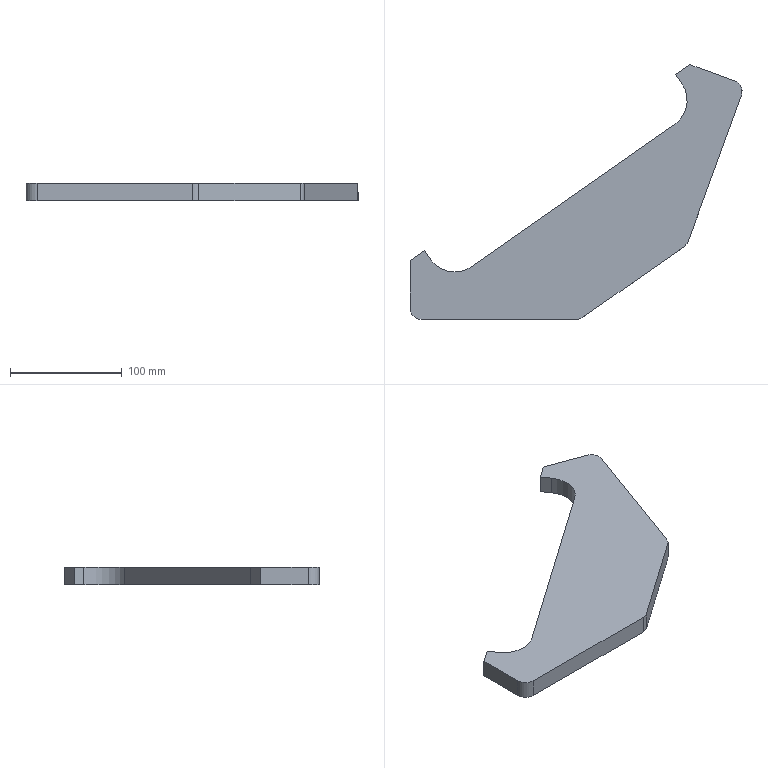Part | SolidWorks | features Extrusion 1, Fillet 1 | 1 solid | 18 faces | box 296.858 x 227.831 x 16 mm | volume 414208 mm3 | plane 12 | cylinder 6 | commonest cylinder face diameters 20 x4 52 x2
STEP:
#1=CARTESIAN_POINT('',(2.583,143.71,16.));
#2=VERTEX_POINT('',#1);
#3=CARTESIAN_POINT('',(93.105,207.095,16.));
#4=VERTEX_POINT('',#3);
#5=CARTESIAN_POINT('',(0.,141.902,16.));
#6=DIRECTION('',(0.8192,0.5736,0.));
#7=VECTOR('',#6,1000.);
#8=LINE('',#5,#7);
#9=EDGE_CURVE('',#2,#4,#8,.T.);
#10=ORIENTED_EDGE('',*,*,#9,.F.);
#11=CARTESIAN_POINT('',(2.583,143.71,0.));
#12=VERTEX_POINT('',#11);
#13=CARTESIAN_POINT('',(2.583,143.71,16.));
#14=DIRECTION('',(0.,0.,-1.));
#15=VECTOR('',#14,1000.);
#16=LINE('',#13,#15);
#17=EDGE_CURVE('',#2,#12,#16,.T.);
#18=ORIENTED_EDGE('',*,*,#17,.T.);
#19=CARTESIAN_POINT('',(93.105,207.095,0.));
#20=VERTEX_POINT('',#19);
#21=CARTESIAN_POINT('',(0.,141.902,0.));
#22=DIRECTION('',(0.8192,0.5736,0.));
#23=VECTOR('',#22,1000.);
#24=LINE('',#21,#23);
#25=EDGE_CURVE('',#12,#20,#24,.T.);
#26=ORIENTED_EDGE('',*,*,#25,.T.);
#27=CARTESIAN_POINT('',(93.105,207.095,16.));
#28=DIRECTION('',(0.,0.,1.));
#29=VECTOR('',#28,1000.);
#30=LINE('',#27,#29);
#31=EDGE_CURVE('',#20,#4,#30,.T.);
#32=ORIENTED_EDGE('',*,*,#31,.T.);
#33=EDGE_LOOP('',(#10,#18,#26,#32));
#34=FACE_OUTER_BOUND('',#33,.T.);
#35=CARTESIAN_POINT('',(0.,141.902,16.));
#36=DIRECTION('',(-0.5736,0.8192,0.));
#37=DIRECTION('',(-0.8192,-0.5736,0.));
#38=AXIS2_PLACEMENT_3D('',#35,#36,#37);
#39=PLANE('',#38);
#40=ADVANCED_FACE('',(#34),#39,.F.);
#41=CARTESIAN_POINT('',(96.767,211.866,16.));
#42=VERTEX_POINT('',#41);
#43=CARTESIAN_POINT('',(144.255,342.34,16.));
#44=VERTEX_POINT('',#43);
#45=CARTESIAN_POINT('',(95.688,208.903,16.));
#46=DIRECTION('',(0.342,0.9397,0.));
#47=VECTOR('',#46,1000.);
#48=LINE('',#45,#47);
#49=EDGE_CURVE('',#42,#44,#48,.T.);
#50=ORIENTED_EDGE('',*,*,#49,.F.);
#51=CARTESIAN_POINT('',(96.767,211.866,0.));
#52=VERTEX_POINT('',#51);
#53=CARTESIAN_POINT('',(96.767,211.866,16.));
#54=DIRECTION('',(0.,0.,-1.));
#55=VECTOR('',#54,1000.);
#56=LINE('',#53,#55);
#57=EDGE_CURVE('',#42,#52,#56,.T.);
#58=ORIENTED_EDGE('',*,*,#57,.T.);
#59=CARTESIAN_POINT('',(144.255,342.34,0.));
#60=VERTEX_POINT('',#59);
#61=CARTESIAN_POINT('',(140.835,332.943,0.));
#62=DIRECTION('',(0.342,0.9397,0.));
#63=VECTOR('',#62,1000.);
#64=LINE('',#61,#63);
#65=EDGE_CURVE('',#52,#60,#64,.T.);
#66=ORIENTED_EDGE('',*,*,#65,.T.);
#67=CARTESIAN_POINT('',(144.255,342.34,16.));
#68=DIRECTION('',(0.,0.,1.));
#69=VECTOR('',#68,1000.);
#70=LINE('',#67,#69);
#71=EDGE_CURVE('',#60,#44,#70,.T.);
#72=ORIENTED_EDGE('',*,*,#71,.T.);
#73=EDGE_LOOP('',(#50,#58,#66,#72));
#74=FACE_OUTER_BOUND('',#73,.T.);
#75=CARTESIAN_POINT('',(140.835,332.943,16.));
#76=DIRECTION('',(-0.9397,0.342,0.));
#77=DIRECTION('',(-0.342,-0.9397,0.));
#78=AXIS2_PLACEMENT_3D('',#75,#76,#77);
#79=PLANE('',#78);
#80=ADVANCED_FACE('',(#74),#79,.F.);
#81=CARTESIAN_POINT('',(138.278,355.157,16.));
#82=VERTEX_POINT('',#81);
#83=CARTESIAN_POINT('',(98.232,369.733,16.));
#84=VERTEX_POINT('',#83);
#85=CARTESIAN_POINT('',(147.675,351.737,16.));
#86=DIRECTION('',(-0.9397,0.342,0.));
#87=VECTOR('',#86,1000.);
#88=LINE('',#85,#87);
#89=EDGE_CURVE('',#82,#84,#88,.T.);
#90=ORIENTED_EDGE('',*,*,#89,.F.);
#91=CARTESIAN_POINT('',(138.278,355.157,0.));
#92=VERTEX_POINT('',#91);
#93=CARTESIAN_POINT('',(138.278,355.157,16.));
#94=DIRECTION('',(0.,0.,-1.));
#95=VECTOR('',#94,1000.);
#96=LINE('',#93,#95);
#97=EDGE_CURVE('',#82,#92,#96,.T.);
#98=ORIENTED_EDGE('',*,*,#97,.T.);
#99=CARTESIAN_POINT('',(98.232,369.733,0.));
#100=VERTEX_POINT('',#99);
#101=CARTESIAN_POINT('',(147.675,351.737,0.));
#102=DIRECTION('',(-0.9397,0.342,0.));
#103=VECTOR('',#102,1000.);
#104=LINE('',#101,#103);
#105=EDGE_CURVE('',#92,#100,#104,.T.);
#106=ORIENTED_EDGE('',*,*,#105,.T.);
#107=CARTESIAN_POINT('',(98.232,369.733,16.));
#108=DIRECTION('',(0.,0.,-1.));
#109=VECTOR('',#108,1000.);
#110=LINE('',#107,#109);
#111=EDGE_CURVE('',#84,#100,#110,.T.);
#112=ORIENTED_EDGE('',*,*,#111,.F.);
#113=EDGE_LOOP('',(#90,#98,#106,#112));
#114=FACE_OUTER_BOUND('',#113,.T.);
#115=CARTESIAN_POINT('',(147.675,351.737,16.));
#116=DIRECTION('',(-0.342,-0.9397,0.));
#117=DIRECTION('',(0.9397,-0.342,0.));
#118=AXIS2_PLACEMENT_3D('',#115,#116,#117);
#119=PLANE('',#118);
#120=ADVANCED_FACE('',(#114),#119,.F.);
#121=CARTESIAN_POINT('',(85.34,360.705,0.));
#122=VERTEX_POINT('',#121);
#123=CARTESIAN_POINT('',(85.34,360.705,0.));
#124=DIRECTION('',(-0.8192,-0.5736,0.));
#125=VECTOR('',#124,1000.);
#126=LINE('',#123,#125);
#127=EDGE_CURVE('',#100,#122,#126,.T.);
#128=ORIENTED_EDGE('',*,*,#127,.T.);
#129=CARTESIAN_POINT('',(85.34,360.705,16.));
#130=VERTEX_POINT('',#129);
#131=CARTESIAN_POINT('',(85.34,360.705,16.));
#132=DIRECTION('',(0.,0.,-1.));
#133=VECTOR('',#132,1000.);
#134=LINE('',#131,#133);
#135=EDGE_CURVE('',#130,#122,#134,.T.);
#136=ORIENTED_EDGE('',*,*,#135,.F.);
#137=CARTESIAN_POINT('',(85.34,360.705,16.));
#138=DIRECTION('',(-0.8192,-0.5736,0.));
#139=VECTOR('',#138,1000.);
#140=LINE('',#137,#139);
#141=EDGE_CURVE('',#84,#130,#140,.T.);
#142=ORIENTED_EDGE('',*,*,#141,.F.);
#143=ORIENTED_EDGE('',*,*,#111,.T.);
#144=EDGE_LOOP('',(#128,#136,#142,#143));
#145=FACE_OUTER_BOUND('',#144,.T.);
#146=CARTESIAN_POINT('',(85.34,360.705,16.));
#147=DIRECTION('',(0.5736,-0.8192,0.));
#148=DIRECTION('',(0.8192,0.5736,0.));
#149=AXIS2_PLACEMENT_3D('',#146,#147,#148);
#150=PLANE('',#149);
#151=ADVANCED_FACE('',(#145),#150,.F.);
#152=CARTESIAN_POINT('',(91.075,352.514,0.));
#153=VERTEX_POINT('',#152);
#154=CARTESIAN_POINT('',(85.34,360.705,0.));
#155=DIRECTION('',(0.5736,-0.8192,0.));
#156=VECTOR('',#155,1000.);
#157=LINE('',#154,#156);
#158=EDGE_CURVE('',#122,#153,#157,.T.);
#159=ORIENTED_EDGE('',*,*,#158,.T.);
#160=CARTESIAN_POINT('',(91.075,352.514,16.));
#161=VERTEX_POINT('',#160);
#162=CARTESIAN_POINT('',(91.075,352.514,16.));
#163=DIRECTION('',(0.,0.,-1.));
#164=VECTOR('',#163,1000.);
#165=LINE('',#162,#164);
#166=EDGE_CURVE('',#161,#153,#165,.T.);
#167=ORIENTED_EDGE('',*,*,#166,.F.);
#168=CARTESIAN_POINT('',(85.34,360.705,16.));
#169=DIRECTION('',(0.5736,-0.8192,0.));
#170=VECTOR('',#169,1000.);
#171=LINE('',#168,#170);
#172=EDGE_CURVE('',#130,#161,#171,.T.);
#173=ORIENTED_EDGE('',*,*,#172,.F.);
#174=ORIENTED_EDGE('',*,*,#135,.T.);
#175=EDGE_LOOP('',(#159,#167,#173,#174));
#176=FACE_OUTER_BOUND('',#175,.T.);
#177=CARTESIAN_POINT('',(85.34,360.705,16.));
#178=DIRECTION('',(0.8192,0.5736,0.));
#179=DIRECTION('',(-0.5736,0.8192,0.));
#180=AXIS2_PLACEMENT_3D('',#177,#178,#179);
#181=PLANE('',#180);
#182=ADVANCED_FACE('',(#176),#181,.F.);
#183=CARTESIAN_POINT('',(84.691,316.303,0.));
#184=VERTEX_POINT('',#183);
#185=CARTESIAN_POINT('',(69.778,337.601,0.));
#186=DIRECTION('',(0.,0.,-1.));
#187=DIRECTION('',(1.,0.,0.));
#188=AXIS2_PLACEMENT_3D('',#185,#186,#187);
#189=CIRCLE('',#188,26.);
#190=EDGE_CURVE('',#153,#184,#189,.T.);
#191=ORIENTED_EDGE('',*,*,#190,.T.);
#192=CARTESIAN_POINT('',(84.691,316.303,16.));
#193=VERTEX_POINT('',#192);
#194=CARTESIAN_POINT('',(84.691,316.303,16.));
#195=DIRECTION('',(0.,0.,-1.));
#196=VECTOR('',#195,1000.);
#197=LINE('',#194,#196);
#198=EDGE_CURVE('',#193,#184,#197,.T.);
#199=ORIENTED_EDGE('',*,*,#198,.F.);
#200=CARTESIAN_POINT('',(69.778,337.601,16.));
#201=DIRECTION('',(0.,0.,-1.));
#202=DIRECTION('',(1.,0.,0.));
#203=AXIS2_PLACEMENT_3D('',#200,#201,#202);
#204=CIRCLE('',#203,26.);
#205=EDGE_CURVE('',#161,#193,#204,.T.);
#206=ORIENTED_EDGE('',*,*,#205,.F.);
#207=ORIENTED_EDGE('',*,*,#166,.T.);
#208=EDGE_LOOP('',(#191,#199,#206,#207));
#209=FACE_OUTER_BOUND('',#208,.T.);
#210=CARTESIAN_POINT('',(69.778,337.601,16.));
#211=DIRECTION('',(0.,0.,-1.));
#212=DIRECTION('',(-1.,0.,0.));
#213=AXIS2_PLACEMENT_3D('',#210,#211,#212);
#214=CYLINDRICAL_SURFACE('',#213,26.);
#215=ADVANCED_FACE('',(#209),#214,.F.);
#216=CARTESIAN_POINT('',(-97.161,188.969,0.));
#217=VERTEX_POINT('',#216);
#218=CARTESIAN_POINT('',(-97.161,188.969,0.));
#219=DIRECTION('',(-0.8192,-0.5736,0.));
#220=VECTOR('',#219,1000.);
#221=LINE('',#218,#220);
#222=EDGE_CURVE('',#184,#217,#221,.T.);
#223=ORIENTED_EDGE('',*,*,#222,.T.);
#224=CARTESIAN_POINT('',(-97.161,188.969,16.));
#225=VERTEX_POINT('',#224);
#226=CARTESIAN_POINT('',(-97.161,188.969,16.));
#227=DIRECTION('',(0.,0.,-1.));
#228=VECTOR('',#227,1000.);
#229=LINE('',#226,#228);
#230=EDGE_CURVE('',#225,#217,#229,.T.);
#231=ORIENTED_EDGE('',*,*,#230,.F.);
#232=CARTESIAN_POINT('',(-97.161,188.969,16.));
#233=DIRECTION('',(-0.8192,-0.5736,0.));
#234=VECTOR('',#233,1000.);
#235=LINE('',#232,#234);
#236=EDGE_CURVE('',#193,#225,#235,.T.);
#237=ORIENTED_EDGE('',*,*,#236,.F.);
#238=ORIENTED_EDGE('',*,*,#198,.T.);
#239=EDGE_LOOP('',(#223,#231,#237,#238));
#240=FACE_OUTER_BOUND('',#239,.T.);
#241=CARTESIAN_POINT('',(-97.161,188.969,16.));
#242=DIRECTION('',(0.5736,-0.8192,0.));
#243=DIRECTION('',(0.8192,0.5736,0.));
#244=AXIS2_PLACEMENT_3D('',#241,#242,#243);
#245=PLANE('',#244);
#246=ADVANCED_FACE('',(#240),#245,.F.);
#247=CARTESIAN_POINT('',(-133.372,195.354,0.));
#248=VERTEX_POINT('',#247);
#249=CARTESIAN_POINT('',(-112.074,210.267,0.));
#250=DIRECTION('',(0.,0.,-1.));
#251=DIRECTION('',(1.,0.,0.));
#252=AXIS2_PLACEMENT_3D('',#249,#250,#251);
#253=CIRCLE('',#252,26.);
#254=EDGE_CURVE('',#217,#248,#253,.T.);
#255=ORIENTED_EDGE('',*,*,#254,.T.);
#256=CARTESIAN_POINT('',(-133.372,195.354,16.));
#257=VERTEX_POINT('',#256);
#258=CARTESIAN_POINT('',(-133.372,195.354,16.));
#259=DIRECTION('',(0.,0.,-1.));
#260=VECTOR('',#259,1000.);
#261=LINE('',#258,#260);
#262=EDGE_CURVE('',#257,#248,#261,.T.);
#263=ORIENTED_EDGE('',*,*,#262,.F.);
#264=CARTESIAN_POINT('',(-112.074,210.267,16.));
#265=DIRECTION('',(0.,0.,-1.));
#266=DIRECTION('',(1.,0.,0.));
#267=AXIS2_PLACEMENT_3D('',#264,#265,#266);
#268=CIRCLE('',#267,26.);
#269=EDGE_CURVE('',#225,#257,#268,.T.);
#270=ORIENTED_EDGE('',*,*,#269,.F.);
#271=ORIENTED_EDGE('',*,*,#230,.T.);
#272=EDGE_LOOP('',(#255,#263,#270,#271));
#273=FACE_OUTER_BOUND('',#272,.T.);
#274=CARTESIAN_POINT('',(-112.074,210.267,16.));
#275=DIRECTION('',(0.,0.,-1.));
#276=DIRECTION('',(-1.,0.,0.));
#277=AXIS2_PLACEMENT_3D('',#274,#275,#276);
#278=CYLINDRICAL_SURFACE('',#277,26.);
#279=ADVANCED_FACE('',(#273),#278,.F.);
#280=CARTESIAN_POINT('',(-139.108,203.546,0.));
#281=VERTEX_POINT('',#280);
#282=CARTESIAN_POINT('',(-133.372,195.354,0.));
#283=DIRECTION('',(-0.5736,0.8192,0.));
#284=VECTOR('',#283,1000.);
#285=LINE('',#282,#284);
#286=EDGE_CURVE('',#248,#281,#285,.T.);
#287=ORIENTED_EDGE('',*,*,#286,.T.);
#288=CARTESIAN_POINT('',(-139.108,203.546,16.));
#289=VERTEX_POINT('',#288);
#290=CARTESIAN_POINT('',(-139.108,203.546,16.));
#291=DIRECTION('',(0.,0.,-1.));
#292=VECTOR('',#291,1000.);
#293=LINE('',#290,#292);
#294=EDGE_CURVE('',#289,#281,#293,.T.);
#295=ORIENTED_EDGE('',*,*,#294,.F.);
#296=CARTESIAN_POINT('',(-133.372,195.354,16.));
#297=DIRECTION('',(-0.5736,0.8192,0.));
#298=VECTOR('',#297,1000.);
#299=LINE('',#296,#298);
#300=EDGE_CURVE('',#257,#289,#299,.T.);
#301=ORIENTED_EDGE('',*,*,#300,.F.);
#302=ORIENTED_EDGE('',*,*,#262,.T.);
#303=EDGE_LOOP('',(#287,#295,#301,#302));
#304=FACE_OUTER_BOUND('',#303,.T.);
#305=CARTESIAN_POINT('',(-133.372,195.354,16.));
#306=DIRECTION('',(-0.8192,-0.5736,0.));
#307=DIRECTION('',(0.5736,-0.8192,0.));
#308=AXIS2_PLACEMENT_3D('',#305,#306,#307);
#309=PLANE('',#308);
#310=ADVANCED_FACE('',(#304),#309,.F.);
#311=CARTESIAN_POINT('',(-152.,194.518,0.));
#312=VERTEX_POINT('',#311);
#313=CARTESIAN_POINT('',(-139.108,203.546,0.));
#314=DIRECTION('',(-0.8192,-0.5736,0.));
#315=VECTOR('',#314,1000.);
#316=LINE('',#313,#315);
#317=EDGE_CURVE('',#281,#312,#316,.T.);
#318=ORIENTED_EDGE('',*,*,#317,.T.);
#319=CARTESIAN_POINT('',(-152.,194.518,16.));
#320=VERTEX_POINT('',#319);
#321=CARTESIAN_POINT('',(-152.,194.518,16.));
#322=DIRECTION('',(0.,0.,-1.));
#323=VECTOR('',#322,1000.);
#324=LINE('',#321,#323);
#325=EDGE_CURVE('',#320,#312,#324,.T.);
#326=ORIENTED_EDGE('',*,*,#325,.F.);
#327=CARTESIAN_POINT('',(-139.108,203.546,16.));
#328=DIRECTION('',(-0.8192,-0.5736,0.));
#329=VECTOR('',#328,1000.);
#330=LINE('',#327,#329);
#331=EDGE_CURVE('',#289,#320,#330,.T.);
#332=ORIENTED_EDGE('',*,*,#331,.F.);
#333=ORIENTED_EDGE('',*,*,#294,.T.);
#334=EDGE_LOOP('',(#318,#326,#332,#333));
#335=FACE_OUTER_BOUND('',#334,.T.);
#336=CARTESIAN_POINT('',(-139.108,203.546,16.));
#337=DIRECTION('',(0.5736,-0.8192,0.));
#338=DIRECTION('',(0.8192,0.5736,0.));
#339=AXIS2_PLACEMENT_3D('',#336,#337,#338);
#340=PLANE('',#339);
#341=ADVANCED_FACE('',(#335),#340,.F.);
#342=CARTESIAN_POINT('',(-152.,151.902,0.));
#343=VERTEX_POINT('',#342);
#344=CARTESIAN_POINT('',(-152.,141.902,0.));
#345=DIRECTION('',(0.,-1.,0.));
#346=VECTOR('',#345,1000.);
#347=LINE('',#344,#346);
#348=EDGE_CURVE('',#312,#343,#347,.T.);
#349=ORIENTED_EDGE('',*,*,#348,.T.);
#350=CARTESIAN_POINT('',(-152.,151.902,16.));
#351=VERTEX_POINT('',#350);
#352=CARTESIAN_POINT('',(-152.,151.902,16.));
#353=DIRECTION('',(0.,0.,1.));
#354=VECTOR('',#353,1000.);
#355=LINE('',#352,#354);
#356=EDGE_CURVE('',#343,#351,#355,.T.);
#357=ORIENTED_EDGE('',*,*,#356,.T.);
#358=CARTESIAN_POINT('',(-152.,141.902,16.));
#359=DIRECTION('',(0.,-1.,0.));
#360=VECTOR('',#359,1000.);
#361=LINE('',#358,#360);
#362=EDGE_CURVE('',#320,#351,#361,.T.);
#363=ORIENTED_EDGE('',*,*,#362,.F.);
#364=ORIENTED_EDGE('',*,*,#325,.T.);
#365=EDGE_LOOP('',(#349,#357,#363,#364));
#366=FACE_OUTER_BOUND('',#365,.T.);
#367=CARTESIAN_POINT('',(-152.,141.902,16.));
#368=DIRECTION('',(1.,0.,0.));
#369=DIRECTION('',(0.,1.,0.));
#370=AXIS2_PLACEMENT_3D('',#367,#368,#369);
#371=PLANE('',#370);
#372=ADVANCED_FACE('',(#366),#371,.F.);
#373=CARTESIAN_POINT('',(-142.,141.902,0.));
#374=VERTEX_POINT('',#373);
#375=CARTESIAN_POINT('',(-3.153,141.902,0.));
#376=VERTEX_POINT('',#375);
#377=CARTESIAN_POINT('',(-132.,141.902,0.));
#378=DIRECTION('',(1.,0.,0.));
#379=VECTOR('',#378,1000.);
#380=LINE('',#377,#379);
#381=EDGE_CURVE('',#374,#376,#380,.T.);
#382=ORIENTED_EDGE('',*,*,#381,.T.);
#383=CARTESIAN_POINT('',(-3.153,141.902,16.));
#384=VERTEX_POINT('',#383);
#385=CARTESIAN_POINT('',(-3.153,141.902,16.));
#386=DIRECTION('',(0.,0.,1.));
#387=VECTOR('',#386,1000.);
#388=LINE('',#385,#387);
#389=EDGE_CURVE('',#376,#384,#388,.T.);
#390=ORIENTED_EDGE('',*,*,#389,.T.);
#391=CARTESIAN_POINT('',(-142.,141.902,16.));
#392=VERTEX_POINT('',#391);
#393=CARTESIAN_POINT('',(-132.,141.902,16.));
#394=DIRECTION('',(1.,0.,0.));
#395=VECTOR('',#394,1000.);
#396=LINE('',#393,#395);
#397=EDGE_CURVE('',#392,#384,#396,.T.);
#398=ORIENTED_EDGE('',*,*,#397,.F.);
#399=CARTESIAN_POINT('',(-142.,141.902,16.));
#400=DIRECTION('',(0.,0.,-1.));
#401=VECTOR('',#400,1000.);
#402=LINE('',#399,#401);
#403=EDGE_CURVE('',#392,#374,#402,.T.);
#404=ORIENTED_EDGE('',*,*,#403,.T.);
#405=EDGE_LOOP('',(#382,#390,#398,#404));
#406=FACE_OUTER_BOUND('',#405,.T.);
#407=CARTESIAN_POINT('',(-132.,141.902,16.));
#408=DIRECTION('',(0.,1.,0.));
#409=DIRECTION('',(-1.,0.,0.));
#410=AXIS2_PLACEMENT_3D('',#407,#408,#409);
#411=PLANE('',#410);
#412=ADVANCED_FACE('',(#406),#411,.F.);
#413=ORIENTED_EDGE('',*,*,#397,.T.);
#414=CARTESIAN_POINT('',(-3.153,151.902,16.));
#415=DIRECTION('',(0.,0.,1.));
#416=DIRECTION('',(1.,0.,0.));
#417=AXIS2_PLACEMENT_3D('',#414,#415,#416);
#418=CIRCLE('',#417,10.);
#419=EDGE_CURVE('',#384,#2,#418,.T.);
#420=ORIENTED_EDGE('',*,*,#419,.T.);
#421=ORIENTED_EDGE('',*,*,#9,.T.);
#422=CARTESIAN_POINT('',(87.37,215.286,16.));
#423=DIRECTION('',(0.,0.,1.));
#424=DIRECTION('',(1.,0.,0.));
#425=AXIS2_PLACEMENT_3D('',#422,#423,#424);
#426=CIRCLE('',#425,10.);
#427=EDGE_CURVE('',#4,#42,#426,.T.);
#428=ORIENTED_EDGE('',*,*,#427,.T.);
#429=ORIENTED_EDGE('',*,*,#49,.T.);
#430=CARTESIAN_POINT('',(134.858,345.76,16.));
#431=DIRECTION('',(0.,0.,1.));
#432=DIRECTION('',(1.,0.,0.));
#433=AXIS2_PLACEMENT_3D('',#430,#431,#432);
#434=CIRCLE('',#433,10.);
#435=EDGE_CURVE('',#44,#82,#434,.T.);
#436=ORIENTED_EDGE('',*,*,#435,.T.);
#437=ORIENTED_EDGE('',*,*,#89,.T.);
#438=ORIENTED_EDGE('',*,*,#141,.T.);
#439=ORIENTED_EDGE('',*,*,#172,.T.);
#440=ORIENTED_EDGE('',*,*,#205,.T.);
#441=ORIENTED_EDGE('',*,*,#236,.T.);
#442=ORIENTED_EDGE('',*,*,#269,.T.);
#443=ORIENTED_EDGE('',*,*,#300,.T.);
#444=ORIENTED_EDGE('',*,*,#331,.T.);
#445=ORIENTED_EDGE('',*,*,#362,.T.);
#446=CARTESIAN_POINT('',(-142.,151.902,16.));
#447=DIRECTION('',(0.,0.,1.));
#448=DIRECTION('',(1.,0.,0.));
#449=AXIS2_PLACEMENT_3D('',#446,#447,#448);
#450=CIRCLE('',#449,10.);
#451=EDGE_CURVE('',#351,#392,#450,.T.);
#452=ORIENTED_EDGE('',*,*,#451,.T.);
#453=EDGE_LOOP('',(#413,#420,#421,#428,#429,#436,#437,#438,#439,#440,#441,#442,#443,#444,#445,#452));
#454=FACE_OUTER_BOUND('',#453,.T.);
#455=CARTESIAN_POINT('',(69.778,337.601,16.));
#456=DIRECTION('',(0.,0.,1.));
#457=DIRECTION('',(1.,0.,0.));
#458=AXIS2_PLACEMENT_3D('',#455,#456,#457);
#459=PLANE('',#458);
#460=ADVANCED_FACE('',(#454),#459,.T.);
#461=ORIENTED_EDGE('',*,*,#25,.F.);
#462=CARTESIAN_POINT('',(-3.153,151.902,0.));
#463=DIRECTION('',(0.,0.,-1.));
#464=DIRECTION('',(1.,0.,0.));
#465=AXIS2_PLACEMENT_3D('',#462,#463,#464);
#466=CIRCLE('',#465,10.);
#467=EDGE_CURVE('',#12,#376,#466,.T.);
#468=ORIENTED_EDGE('',*,*,#467,.T.);
#469=ORIENTED_EDGE('',*,*,#381,.F.);
#470=CARTESIAN_POINT('',(-142.,151.902,0.));
#471=DIRECTION('',(0.,0.,-1.));
#472=DIRECTION('',(1.,0.,0.));
#473=AXIS2_PLACEMENT_3D('',#470,#471,#472);
#474=CIRCLE('',#473,10.);
#475=EDGE_CURVE('',#374,#343,#474,.T.);
#476=ORIENTED_EDGE('',*,*,#475,.T.);
#477=ORIENTED_EDGE('',*,*,#348,.F.);
#478=ORIENTED_EDGE('',*,*,#317,.F.);
#479=ORIENTED_EDGE('',*,*,#286,.F.);
#480=ORIENTED_EDGE('',*,*,#254,.F.);
#481=ORIENTED_EDGE('',*,*,#222,.F.);
#482=ORIENTED_EDGE('',*,*,#190,.F.);
#483=ORIENTED_EDGE('',*,*,#158,.F.);
#484=ORIENTED_EDGE('',*,*,#127,.F.);
#485=ORIENTED_EDGE('',*,*,#105,.F.);
#486=CARTESIAN_POINT('',(134.858,345.76,0.));
#487=DIRECTION('',(0.,0.,-1.));
#488=DIRECTION('',(1.,0.,0.));
#489=AXIS2_PLACEMENT_3D('',#486,#487,#488);
#490=CIRCLE('',#489,10.);
#491=EDGE_CURVE('',#92,#60,#490,.T.);
#492=ORIENTED_EDGE('',*,*,#491,.T.);
#493=ORIENTED_EDGE('',*,*,#65,.F.);
#494=CARTESIAN_POINT('',(87.37,215.286,0.));
#495=DIRECTION('',(0.,0.,-1.));
#496=DIRECTION('',(1.,0.,0.));
#497=AXIS2_PLACEMENT_3D('',#494,#495,#496);
#498=CIRCLE('',#497,10.);
#499=EDGE_CURVE('',#52,#20,#498,.T.);
#500=ORIENTED_EDGE('',*,*,#499,.T.);
#501=EDGE_LOOP('',(#461,#468,#469,#476,#477,#478,#479,#480,#481,#482,#483,#484,#485,#492,#493,#500));
#502=FACE_OUTER_BOUND('',#501,.T.);
#503=CARTESIAN_POINT('',(69.778,337.601,0.));
#504=DIRECTION('',(0.,0.,1.));
#505=DIRECTION('',(1.,0.,0.));
#506=AXIS2_PLACEMENT_3D('',#503,#504,#505);
#507=PLANE('',#506);
#508=ADVANCED_FACE('',(#502),#507,.F.);
#509=ORIENTED_EDGE('',*,*,#419,.F.);
#510=ORIENTED_EDGE('',*,*,#389,.F.);
#511=ORIENTED_EDGE('',*,*,#467,.F.);
#512=ORIENTED_EDGE('',*,*,#17,.F.);
#513=EDGE_LOOP('',(#509,#510,#511,#512));
#514=FACE_OUTER_BOUND('',#513,.T.);
#515=CARTESIAN_POINT('',(-3.153,151.902,16.));
#516=DIRECTION('',(0.,0.,-1.));
#517=DIRECTION('',(-1.,0.,0.));
#518=AXIS2_PLACEMENT_3D('',#515,#516,#517);
#519=CYLINDRICAL_SURFACE('',#518,10.);
#520=ADVANCED_FACE('',(#514),#519,.T.);
#521=ORIENTED_EDGE('',*,*,#427,.F.);
#522=ORIENTED_EDGE('',*,*,#31,.F.);
#523=ORIENTED_EDGE('',*,*,#499,.F.);
#524=ORIENTED_EDGE('',*,*,#57,.F.);
#525=EDGE_LOOP('',(#521,#522,#523,#524));
#526=FACE_OUTER_BOUND('',#525,.T.);
#527=CARTESIAN_POINT('',(87.37,215.286,16.));
#528=DIRECTION('',(0.,0.,-1.));
#529=DIRECTION('',(-1.,0.,0.));
#530=AXIS2_PLACEMENT_3D('',#527,#528,#529);
#531=CYLINDRICAL_SURFACE('',#530,10.);
#532=ADVANCED_FACE('',(#526),#531,.T.);
#533=ORIENTED_EDGE('',*,*,#451,.F.);
#534=ORIENTED_EDGE('',*,*,#356,.F.);
#535=ORIENTED_EDGE('',*,*,#475,.F.);
#536=ORIENTED_EDGE('',*,*,#403,.F.);
#537=EDGE_LOOP('',(#533,#534,#535,#536));
#538=FACE_OUTER_BOUND('',#537,.T.);
#539=CARTESIAN_POINT('',(-142.,151.902,16.));
#540=DIRECTION('',(0.,0.,-1.));
#541=DIRECTION('',(-1.,0.,0.));
#542=AXIS2_PLACEMENT_3D('',#539,#540,#541);
#543=CYLINDRICAL_SURFACE('',#542,10.);
#544=ADVANCED_FACE('',(#538),#543,.T.);
#545=ORIENTED_EDGE('',*,*,#435,.F.);
#546=ORIENTED_EDGE('',*,*,#71,.F.);
#547=ORIENTED_EDGE('',*,*,#491,.F.);
#548=ORIENTED_EDGE('',*,*,#97,.F.);
#549=EDGE_LOOP('',(#545,#546,#547,#548));
#550=FACE_OUTER_BOUND('',#549,.T.);
#551=CARTESIAN_POINT('',(134.858,345.76,16.));
#552=DIRECTION('',(0.,0.,-1.));
#553=DIRECTION('',(-1.,0.,0.));
#554=AXIS2_PLACEMENT_3D('',#551,#552,#553);
#555=CYLINDRICAL_SURFACE('',#554,10.);
#556=ADVANCED_FACE('',(#550),#555,.T.);
#557=CLOSED_SHELL('',(#40,#80,#120,#151,#182,#215,#246,#279,#310,#341,#372,#412,#460,#508,#520,#532,#544,#556));
#558=MANIFOLD_SOLID_BREP('',#557);
#559=CARTESIAN_POINT('',(0.,0.,0.));
#560=DIRECTION('',(0.,0.,1.));
#561=DIRECTION('',(1.,0.,0.));
#562=AXIS2_PLACEMENT_3D('',#559,#560,#561);
#563=(LENGTH_UNIT()NAMED_UNIT(*)SI_UNIT(.MILLI.,.METRE.));
#564=UNCERTAINTY_MEASURE_WITH_UNIT(LENGTH_MEASURE(0.00001),#563,'','');
#565=(NAMED_UNIT(*)PLANE_ANGLE_UNIT()SI_UNIT($,.RADIAN.));
#566=(NAMED_UNIT(*)SI_UNIT($,.STERADIAN.)SOLID_ANGLE_UNIT());
#567=(GEOMETRIC_REPRESENTATION_CONTEXT(3)GLOBAL_UNCERTAINTY_ASSIGNED_CONTEXT((#564))GLOBAL_UNIT_ASSIGNED_CONTEXT((#563,#565,#566))REPRESENTATION_CONTEXT('',''));
#568=ADVANCED_BREP_SHAPE_REPRESENTATION('',(#558,#562),#567);